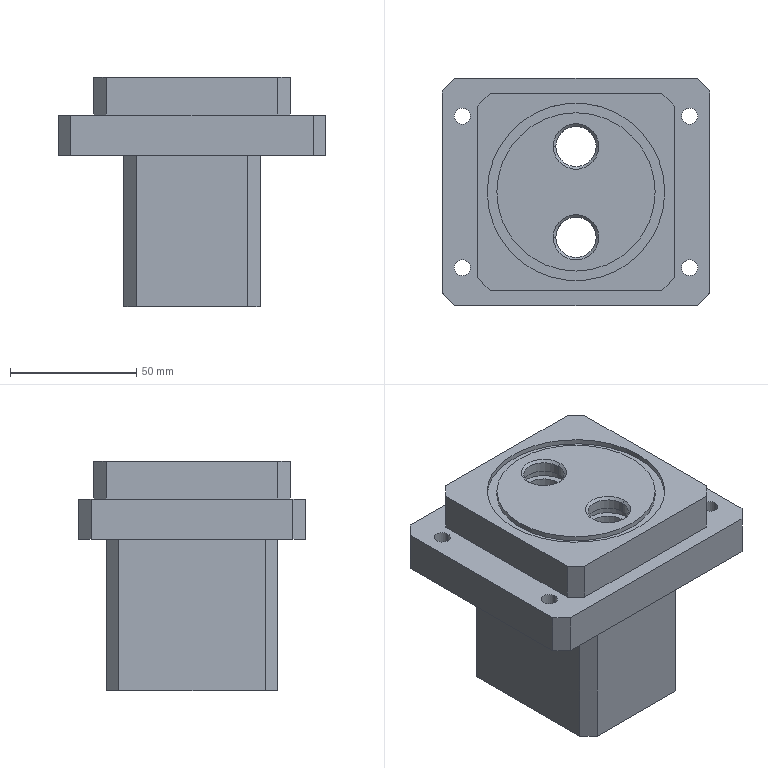Part | SolidWorks | features HoleWzd 4, ICE 4, Chamfer 2, Extrusion 1 | 1 solid | 100 faces | box 106 x 90 x 91 mm | volume 392922 mm3 | cylinder 44 | plane 40 | cone 16 | commonest cylinder face diameters 4.2 x8 6.4 x8 11 x8 16 x8 20.6 x4 22 x4